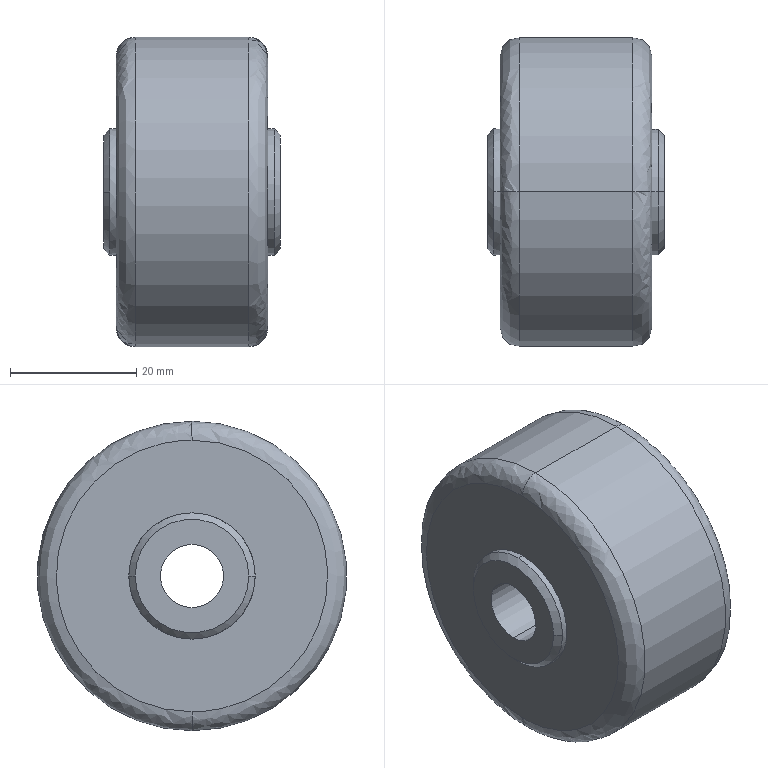Part | STEP file | HI_CGR51-60-U-001 | 1 solid | 20 faces | box 28 x 49 x 49 mm | volume 43678 mm3 | cylinder 8 | spline 4 | cone 4 | plane 4 | commonest cylinder face diameters 20 x4 10 x2 49 x2